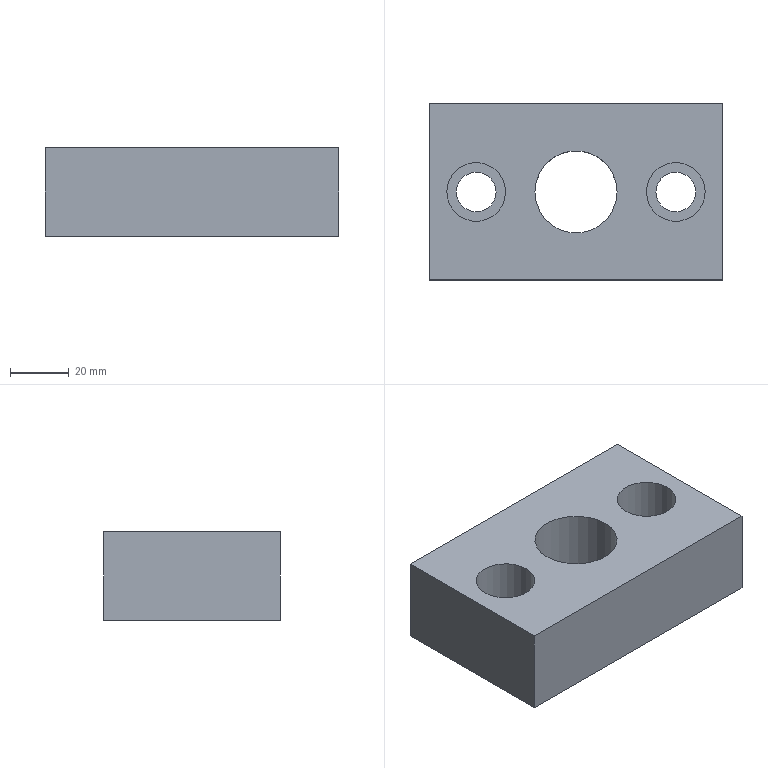Part | STEP file | lll_id4842_x_t | 1 solid | 15 faces | box 100 x 60 x 30 mm | volume 143309 mm3 | plane 9 | cylinder 6 | commonest cylinder face diameters 13.509 x2 20.008 x2 28 x1 40 x1
STEP:
#1=CARTESIAN_POINT('',(2246.,160.,-50.));
#2=VERTEX_POINT('',#1);
#3=CARTESIAN_POINT('',(2260.,160.,-50.));
#4=DIRECTION('',(0.,0.,1.));
#5=DIRECTION('',(-1.,0.,0.));
#6=AXIS2_PLACEMENT_3D('',#3,#4,#5);
#7=CIRCLE('',#6,14.);
#8=EDGE_CURVE('',#2,#2,#7,.T.);
#9=ORIENTED_EDGE('',*,*,#8,.F.);
#10=EDGE_LOOP('',(#9));
#11=FACE_BOUND('',#10,.T.);
#12=CARTESIAN_POINT('',(2283.996,160.,-50.));
#13=VERTEX_POINT('',#12);
#14=CARTESIAN_POINT('',(2294.,160.,-50.));
#15=DIRECTION('',(0.,0.,-1.));
#16=DIRECTION('',(-1.,0.,0.));
#17=AXIS2_PLACEMENT_3D('',#14,#15,#16);
#18=CIRCLE('',#17,10.004);
#19=EDGE_CURVE('',#13,#13,#18,.T.);
#20=ORIENTED_EDGE('',*,*,#19,.T.);
#21=EDGE_LOOP('',(#20));
#22=FACE_BOUND('',#21,.T.);
#23=CARTESIAN_POINT('',(2210.,190.,-50.));
#24=VERTEX_POINT('',#23);
#25=CARTESIAN_POINT('',(2310.,190.,-50.));
#26=VERTEX_POINT('',#25);
#27=CARTESIAN_POINT('',(2260.,190.,-50.));
#28=DIRECTION('',(1.,0.,0.));
#29=VECTOR('',#28,1.);
#30=LINE('',#27,#29);
#31=EDGE_CURVE('',#24,#26,#30,.T.);
#32=ORIENTED_EDGE('',*,*,#31,.F.);
#33=CARTESIAN_POINT('',(2210.,130.,-50.));
#34=VERTEX_POINT('',#33);
#35=CARTESIAN_POINT('',(2210.,160.,-50.));
#36=DIRECTION('',(0.,1.,0.));
#37=VECTOR('',#36,1.);
#38=LINE('',#35,#37);
#39=EDGE_CURVE('',#34,#24,#38,.T.);
#40=ORIENTED_EDGE('',*,*,#39,.F.);
#41=CARTESIAN_POINT('',(2310.,130.,-50.));
#42=VERTEX_POINT('',#41);
#43=CARTESIAN_POINT('',(2260.,130.,-50.));
#44=DIRECTION('',(-1.,0.,0.));
#45=VECTOR('',#44,1.);
#46=LINE('',#43,#45);
#47=EDGE_CURVE('',#42,#34,#46,.T.);
#48=ORIENTED_EDGE('',*,*,#47,.F.);
#49=CARTESIAN_POINT('',(2310.,160.,-50.));
#50=DIRECTION('',(0.,-1.,0.));
#51=VECTOR('',#50,1.);
#52=LINE('',#49,#51);
#53=EDGE_CURVE('',#26,#42,#52,.T.);
#54=ORIENTED_EDGE('',*,*,#53,.F.);
#55=EDGE_LOOP('',(#32,#40,#48,#54));
#56=FACE_BOUND('',#55,.T.);
#57=CARTESIAN_POINT('',(2215.996,160.,-50.));
#58=VERTEX_POINT('',#57);
#59=CARTESIAN_POINT('',(2226.,160.,-50.));
#60=DIRECTION('',(0.,0.,-1.));
#61=DIRECTION('',(-1.,0.,0.));
#62=AXIS2_PLACEMENT_3D('',#59,#60,#61);
#63=CIRCLE('',#62,10.004);
#64=EDGE_CURVE('',#58,#58,#63,.T.);
#65=ORIENTED_EDGE('',*,*,#64,.T.);
#66=EDGE_LOOP('',(#65));
#67=FACE_BOUND('',#66,.T.);
#68=CARTESIAN_POINT('',(2260.,160.,-50.));
#69=DIRECTION('',(0.,0.,1.));
#70=DIRECTION('',(-1.,0.,0.));
#71=AXIS2_PLACEMENT_3D('',#68,#69,#70);
#72=PLANE('',#71);
#73=ADVANCED_FACE('',(#11,#22,#56,#67),#72,.T.);
#74=CARTESIAN_POINT('',(2210.,190.,-80.));
#75=VERTEX_POINT('',#74);
#76=CARTESIAN_POINT('',(2210.,190.,-80.));
#77=DIRECTION('',(0.,0.,1.));
#78=VECTOR('',#77,1.);
#79=LINE('',#76,#78);
#80=EDGE_CURVE('',#75,#24,#79,.T.);
#81=ORIENTED_EDGE('',*,*,#80,.T.);
#82=ORIENTED_EDGE('',*,*,#31,.T.);
#83=CARTESIAN_POINT('',(2310.,190.,-80.));
#84=VERTEX_POINT('',#83);
#85=CARTESIAN_POINT('',(2310.,190.,-80.));
#86=DIRECTION('',(0.,0.,1.));
#87=VECTOR('',#86,1.);
#88=LINE('',#85,#87);
#89=EDGE_CURVE('',#84,#26,#88,.T.);
#90=ORIENTED_EDGE('',*,*,#89,.F.);
#91=CARTESIAN_POINT('',(2260.,190.,-80.));
#92=DIRECTION('',(-1.,0.,0.));
#93=VECTOR('',#92,1.);
#94=LINE('',#91,#93);
#95=EDGE_CURVE('',#84,#75,#94,.T.);
#96=ORIENTED_EDGE('',*,*,#95,.T.);
#97=EDGE_LOOP('',(#81,#82,#90,#96));
#98=FACE_OUTER_BOUND('',#97,.T.);
#99=CARTESIAN_POINT('',(2260.,190.,-80.));
#100=DIRECTION('',(0.,1.,0.));
#101=DIRECTION('',(0.,0.,-1.));
#102=AXIS2_PLACEMENT_3D('',#99,#100,#101);
#103=PLANE('',#102);
#104=ADVANCED_FACE('',(#98),#103,.T.);
#105=ORIENTED_EDGE('',*,*,#89,.T.);
#106=ORIENTED_EDGE('',*,*,#53,.T.);
#107=CARTESIAN_POINT('',(2310.,130.,-80.));
#108=VERTEX_POINT('',#107);
#109=CARTESIAN_POINT('',(2310.,130.,-80.));
#110=DIRECTION('',(0.,0.,1.));
#111=VECTOR('',#110,1.);
#112=LINE('',#109,#111);
#113=EDGE_CURVE('',#108,#42,#112,.T.);
#114=ORIENTED_EDGE('',*,*,#113,.F.);
#115=CARTESIAN_POINT('',(2310.,160.,-80.));
#116=DIRECTION('',(0.,1.,0.));
#117=VECTOR('',#116,1.);
#118=LINE('',#115,#117);
#119=EDGE_CURVE('',#108,#84,#118,.T.);
#120=ORIENTED_EDGE('',*,*,#119,.T.);
#121=EDGE_LOOP('',(#105,#106,#114,#120));
#122=FACE_OUTER_BOUND('',#121,.T.);
#123=CARTESIAN_POINT('',(2310.,160.,-80.));
#124=DIRECTION('',(1.,0.,0.));
#125=DIRECTION('',(0.,0.,1.));
#126=AXIS2_PLACEMENT_3D('',#123,#124,#125);
#127=PLANE('',#126);
#128=ADVANCED_FACE('',(#122),#127,.T.);
#129=ORIENTED_EDGE('',*,*,#113,.T.);
#130=ORIENTED_EDGE('',*,*,#47,.T.);
#131=CARTESIAN_POINT('',(2210.,130.,-80.));
#132=VERTEX_POINT('',#131);
#133=CARTESIAN_POINT('',(2210.,130.,-80.));
#134=DIRECTION('',(0.,0.,1.));
#135=VECTOR('',#134,1.);
#136=LINE('',#133,#135);
#137=EDGE_CURVE('',#132,#34,#136,.T.);
#138=ORIENTED_EDGE('',*,*,#137,.F.);
#139=CARTESIAN_POINT('',(2260.,130.,-80.));
#140=DIRECTION('',(1.,0.,0.));
#141=VECTOR('',#140,1.);
#142=LINE('',#139,#141);
#143=EDGE_CURVE('',#132,#108,#142,.T.);
#144=ORIENTED_EDGE('',*,*,#143,.T.);
#145=EDGE_LOOP('',(#129,#130,#138,#144));
#146=FACE_OUTER_BOUND('',#145,.T.);
#147=CARTESIAN_POINT('',(2260.,130.,-80.));
#148=DIRECTION('',(0.,-1.,0.));
#149=DIRECTION('',(0.,0.,1.));
#150=AXIS2_PLACEMENT_3D('',#147,#148,#149);
#151=PLANE('',#150);
#152=ADVANCED_FACE('',(#146),#151,.T.);
#153=CARTESIAN_POINT('',(2232.755,160.,-80.));
#154=VERTEX_POINT('',#153);
#155=CARTESIAN_POINT('',(2226.,160.,-80.));
#156=DIRECTION('',(0.,0.,-1.));
#157=DIRECTION('',(1.,0.,0.));
#158=AXIS2_PLACEMENT_3D('',#155,#156,#157);
#159=CIRCLE('',#158,6.755);
#160=EDGE_CURVE('',#154,#154,#159,.T.);
#161=ORIENTED_EDGE('',*,*,#160,.F.);
#162=EDGE_LOOP('',(#161));
#163=FACE_BOUND('',#162,.T.);
#164=CARTESIAN_POINT('',(2300.755,160.,-80.));
#165=VERTEX_POINT('',#164);
#166=CARTESIAN_POINT('',(2294.,160.,-80.));
#167=DIRECTION('',(0.,0.,-1.));
#168=DIRECTION('',(1.,0.,0.));
#169=AXIS2_PLACEMENT_3D('',#166,#167,#168);
#170=CIRCLE('',#169,6.755);
#171=EDGE_CURVE('',#165,#165,#170,.T.);
#172=ORIENTED_EDGE('',*,*,#171,.F.);
#173=EDGE_LOOP('',(#172));
#174=FACE_BOUND('',#173,.T.);
#175=CARTESIAN_POINT('',(2280.,160.,-80.));
#176=VERTEX_POINT('',#175);
#177=CARTESIAN_POINT('',(2260.,160.,-80.));
#178=DIRECTION('',(0.,0.,-1.));
#179=DIRECTION('',(1.,0.,0.));
#180=AXIS2_PLACEMENT_3D('',#177,#178,#179);
#181=CIRCLE('',#180,20.);
#182=EDGE_CURVE('',#176,#176,#181,.T.);
#183=ORIENTED_EDGE('',*,*,#182,.F.);
#184=EDGE_LOOP('',(#183));
#185=FACE_BOUND('',#184,.T.);
#186=CARTESIAN_POINT('',(2210.,160.,-80.));
#187=DIRECTION('',(0.,-1.,0.));
#188=VECTOR('',#187,1.);
#189=LINE('',#186,#188);
#190=EDGE_CURVE('',#75,#132,#189,.T.);
#191=ORIENTED_EDGE('',*,*,#190,.F.);
#192=ORIENTED_EDGE('',*,*,#95,.F.);
#193=ORIENTED_EDGE('',*,*,#119,.F.);
#194=ORIENTED_EDGE('',*,*,#143,.F.);
#195=EDGE_LOOP('',(#191,#192,#193,#194));
#196=FACE_BOUND('',#195,.T.);
#197=CARTESIAN_POINT('',(2260.,160.,-80.));
#198=DIRECTION('',(0.,0.,-1.));
#199=DIRECTION('',(1.,0.,0.));
#200=AXIS2_PLACEMENT_3D('',#197,#198,#199);
#201=PLANE('',#200);
#202=ADVANCED_FACE('',(#163,#174,#185,#196),#201,.T.);
#203=ORIENTED_EDGE('',*,*,#190,.T.);
#204=ORIENTED_EDGE('',*,*,#137,.T.);
#205=ORIENTED_EDGE('',*,*,#39,.T.);
#206=ORIENTED_EDGE('',*,*,#80,.F.);
#207=EDGE_LOOP('',(#203,#204,#205,#206));
#208=FACE_OUTER_BOUND('',#207,.T.);
#209=CARTESIAN_POINT('',(2210.,160.,-80.));
#210=DIRECTION('',(-1.,0.,0.));
#211=DIRECTION('',(0.,0.,-1.));
#212=AXIS2_PLACEMENT_3D('',#209,#210,#211);
#213=PLANE('',#212);
#214=ADVANCED_FACE('',(#208),#213,.T.);
#215=CARTESIAN_POINT('',(2246.,160.,-73.));
#216=VERTEX_POINT('',#215);
#217=CARTESIAN_POINT('',(2260.,160.,-73.));
#218=DIRECTION('',(0.,0.,1.));
#219=DIRECTION('',(1.,0.,0.));
#220=AXIS2_PLACEMENT_3D('',#217,#218,#219);
#221=CIRCLE('',#220,14.);
#222=EDGE_CURVE('',#216,#216,#221,.T.);
#223=ORIENTED_EDGE('',*,*,#222,.T.);
#224=EDGE_LOOP('',(#223));
#225=FACE_BOUND('',#224,.T.);
#226=CARTESIAN_POINT('',(2240.,160.,-73.));
#227=VERTEX_POINT('',#226);
#228=CARTESIAN_POINT('',(2260.,160.,-73.));
#229=DIRECTION('',(0.,0.,1.));
#230=DIRECTION('',(1.,0.,0.));
#231=AXIS2_PLACEMENT_3D('',#228,#229,#230);
#232=CIRCLE('',#231,20.);
#233=EDGE_CURVE('',#227,#227,#232,.T.);
#234=ORIENTED_EDGE('',*,*,#233,.F.);
#235=EDGE_LOOP('',(#234));
#236=FACE_BOUND('',#235,.T.);
#237=CARTESIAN_POINT('',(2260.,160.,-73.));
#238=DIRECTION('',(0.,0.,1.));
#239=DIRECTION('',(-1.,0.,0.));
#240=AXIS2_PLACEMENT_3D('',#237,#238,#239);
#241=PLANE('',#240);
#242=ADVANCED_FACE('',(#225,#236),#241,.F.);
#243=ORIENTED_EDGE('',*,*,#182,.T.);
#244=EDGE_LOOP('',(#243));
#245=FACE_BOUND('',#244,.T.);
#246=ORIENTED_EDGE('',*,*,#233,.T.);
#247=EDGE_LOOP('',(#246));
#248=FACE_BOUND('',#247,.T.);
#249=CARTESIAN_POINT('',(2260.,160.,-75.));
#250=DIRECTION('',(0.,0.,-1.));
#251=DIRECTION('',(-1.,0.,0.));
#252=AXIS2_PLACEMENT_3D('',#249,#250,#251);
#253=CYLINDRICAL_SURFACE('',#252,20.);
#254=ADVANCED_FACE('',(#245,#248),#253,.F.);
#255=ORIENTED_EDGE('',*,*,#171,.T.);
#256=EDGE_LOOP('',(#255));
#257=FACE_BOUND('',#256,.T.);
#258=CARTESIAN_POINT('',(2300.755,160.,-65.));
#259=VERTEX_POINT('',#258);
#260=CARTESIAN_POINT('',(2294.,160.,-65.));
#261=DIRECTION('',(0.,0.,-1.));
#262=DIRECTION('',(1.,0.,0.));
#263=AXIS2_PLACEMENT_3D('',#260,#261,#262);
#264=CIRCLE('',#263,6.755);
#265=EDGE_CURVE('',#259,#259,#264,.T.);
#266=ORIENTED_EDGE('',*,*,#265,.F.);
#267=EDGE_LOOP('',(#266));
#268=FACE_BOUND('',#267,.T.);
#269=CARTESIAN_POINT('',(2294.,160.,-48.));
#270=DIRECTION('',(0.,0.,-1.));
#271=DIRECTION('',(-1.,0.,0.));
#272=AXIS2_PLACEMENT_3D('',#269,#270,#271);
#273=CYLINDRICAL_SURFACE('',#272,6.755);
#274=ADVANCED_FACE('',(#257,#268),#273,.F.);
#275=ORIENTED_EDGE('',*,*,#265,.T.);
#276=EDGE_LOOP('',(#275));
#277=FACE_BOUND('',#276,.T.);
#278=CARTESIAN_POINT('',(2283.996,160.,-65.));
#279=VERTEX_POINT('',#278);
#280=CARTESIAN_POINT('',(2294.,160.,-65.));
#281=DIRECTION('',(0.,0.,-1.));
#282=DIRECTION('',(-1.,0.,0.));
#283=AXIS2_PLACEMENT_3D('',#280,#281,#282);
#284=CIRCLE('',#283,10.004);
#285=EDGE_CURVE('',#279,#279,#284,.T.);
#286=ORIENTED_EDGE('',*,*,#285,.F.);
#287=EDGE_LOOP('',(#286));
#288=FACE_BOUND('',#287,.T.);
#289=CARTESIAN_POINT('',(2294.,160.,-65.));
#290=DIRECTION('',(0.,0.,-1.));
#291=DIRECTION('',(1.,0.,0.));
#292=AXIS2_PLACEMENT_3D('',#289,#290,#291);
#293=PLANE('',#292);
#294=ADVANCED_FACE('',(#277,#288),#293,.F.);
#295=ORIENTED_EDGE('',*,*,#285,.T.);
#296=EDGE_LOOP('',(#295));
#297=FACE_BOUND('',#296,.T.);
#298=ORIENTED_EDGE('',*,*,#19,.F.);
#299=EDGE_LOOP('',(#298));
#300=FACE_BOUND('',#299,.T.);
#301=CARTESIAN_POINT('',(2294.,160.,-50.));
#302=DIRECTION('',(0.,0.,-1.));
#303=DIRECTION('',(-1.,0.,0.));
#304=AXIS2_PLACEMENT_3D('',#301,#302,#303);
#305=CYLINDRICAL_SURFACE('',#304,10.004);
#306=ADVANCED_FACE('',(#297,#300),#305,.F.);
#307=ORIENTED_EDGE('',*,*,#160,.T.);
#308=EDGE_LOOP('',(#307));
#309=FACE_BOUND('',#308,.T.);
#310=CARTESIAN_POINT('',(2232.755,160.,-65.));
#311=VERTEX_POINT('',#310);
#312=CARTESIAN_POINT('',(2226.,160.,-65.));
#313=DIRECTION('',(0.,0.,-1.));
#314=DIRECTION('',(1.,0.,0.));
#315=AXIS2_PLACEMENT_3D('',#312,#313,#314);
#316=CIRCLE('',#315,6.755);
#317=EDGE_CURVE('',#311,#311,#316,.T.);
#318=ORIENTED_EDGE('',*,*,#317,.F.);
#319=EDGE_LOOP('',(#318));
#320=FACE_BOUND('',#319,.T.);
#321=CARTESIAN_POINT('',(2226.,160.,-48.));
#322=DIRECTION('',(0.,0.,-1.));
#323=DIRECTION('',(-1.,0.,0.));
#324=AXIS2_PLACEMENT_3D('',#321,#322,#323);
#325=CYLINDRICAL_SURFACE('',#324,6.755);
#326=ADVANCED_FACE('',(#309,#320),#325,.F.);
#327=ORIENTED_EDGE('',*,*,#317,.T.);
#328=EDGE_LOOP('',(#327));
#329=FACE_BOUND('',#328,.T.);
#330=CARTESIAN_POINT('',(2215.996,160.,-65.));
#331=VERTEX_POINT('',#330);
#332=CARTESIAN_POINT('',(2226.,160.,-65.));
#333=DIRECTION('',(0.,0.,-1.));
#334=DIRECTION('',(-1.,0.,0.));
#335=AXIS2_PLACEMENT_3D('',#332,#333,#334);
#336=CIRCLE('',#335,10.004);
#337=EDGE_CURVE('',#331,#331,#336,.T.);
#338=ORIENTED_EDGE('',*,*,#337,.F.);
#339=EDGE_LOOP('',(#338));
#340=FACE_BOUND('',#339,.T.);
#341=CARTESIAN_POINT('',(2226.,160.,-65.));
#342=DIRECTION('',(0.,0.,-1.));
#343=DIRECTION('',(1.,0.,0.));
#344=AXIS2_PLACEMENT_3D('',#341,#342,#343);
#345=PLANE('',#344);
#346=ADVANCED_FACE('',(#329,#340),#345,.F.);
#347=ORIENTED_EDGE('',*,*,#337,.T.);
#348=EDGE_LOOP('',(#347));
#349=FACE_BOUND('',#348,.T.);
#350=ORIENTED_EDGE('',*,*,#64,.F.);
#351=EDGE_LOOP('',(#350));
#352=FACE_BOUND('',#351,.T.);
#353=CARTESIAN_POINT('',(2226.,160.,-50.));
#354=DIRECTION('',(0.,0.,-1.));
#355=DIRECTION('',(-1.,0.,0.));
#356=AXIS2_PLACEMENT_3D('',#353,#354,#355);
#357=CYLINDRICAL_SURFACE('',#356,10.004);
#358=ADVANCED_FACE('',(#349,#352),#357,.F.);
#359=ORIENTED_EDGE('',*,*,#8,.T.);
#360=EDGE_LOOP('',(#359));
#361=FACE_BOUND('',#360,.T.);
#362=ORIENTED_EDGE('',*,*,#222,.F.);
#363=EDGE_LOOP('',(#362));
#364=FACE_BOUND('',#363,.T.);
#365=CARTESIAN_POINT('',(2260.,160.,-8.));
#366=DIRECTION('',(0.,0.,-1.));
#367=DIRECTION('',(-1.,0.,0.));
#368=AXIS2_PLACEMENT_3D('',#365,#366,#367);
#369=CYLINDRICAL_SURFACE('',#368,14.);
#370=ADVANCED_FACE('',(#361,#364),#369,.F.);
#371=CLOSED_SHELL('',(#73,#104,#128,#152,#202,#214,#242,#254,#274,#294,#306,#326,#346,#358,#370));
#372=MANIFOLD_SOLID_BREP('',#371);
#373=(LENGTH_UNIT()NAMED_UNIT(*)SI_UNIT(.MILLI.,.METRE.));
#374=UNCERTAINTY_MEASURE_WITH_UNIT(LENGTH_MEASURE(0.00002),#373,'','');
#375=(NAMED_UNIT(*)PLANE_ANGLE_UNIT()SI_UNIT($,.RADIAN.));
#376=PLANE_ANGLE_MEASURE_WITH_UNIT(PLANE_ANGLE_MEASURE(0.01745),#375);
#377=DIMENSIONAL_EXPONENTS(0.,0.,0.,0.,0.,0.,0.);
#378=(CONVERSION_BASED_UNIT('DEGREE',#376)NAMED_UNIT(#377)PLANE_ANGLE_UNIT());
#379=(NAMED_UNIT(*)SI_UNIT($,.STERADIAN.)SOLID_ANGLE_UNIT());
#380=(GEOMETRIC_REPRESENTATION_CONTEXT(3)GLOBAL_UNCERTAINTY_ASSIGNED_CONTEXT((#374))GLOBAL_UNIT_ASSIGNED_CONTEXT((#373,#378,#379))REPRESENTATION_CONTEXT('',''));
#381=ADVANCED_BREP_SHAPE_REPRESENTATION('',(#372),#380);